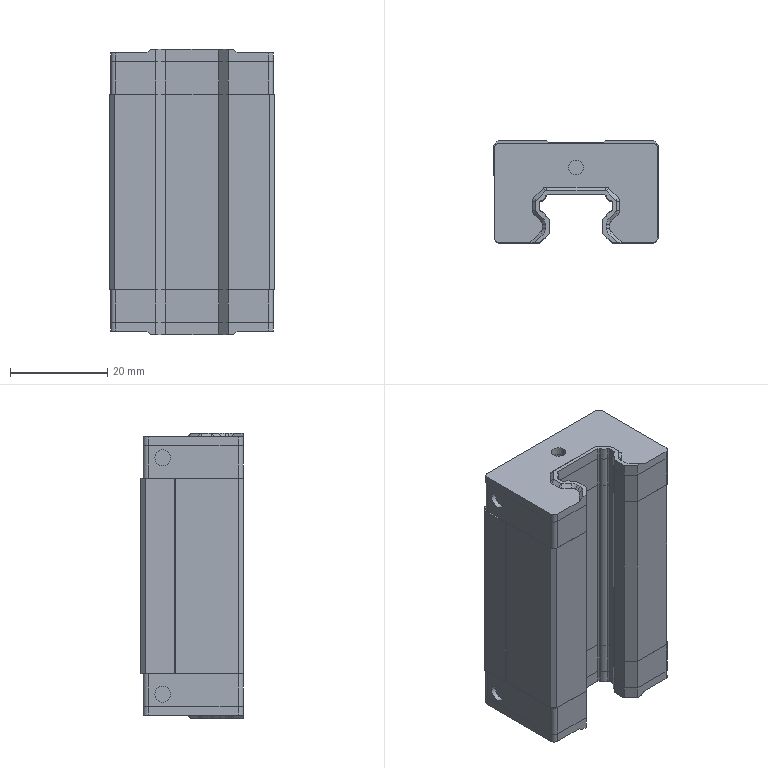Part | SolidWorks | 5 solids | 276 faces | box 34 x 21 x 58.6 mm | volume 32343 mm3 | plane 132 | cylinder 108 | cone 36 | commonest cylinder face diameters 0.6 x40 2.6 x20 3.3 x20 2 x16 4 x8 3 x4